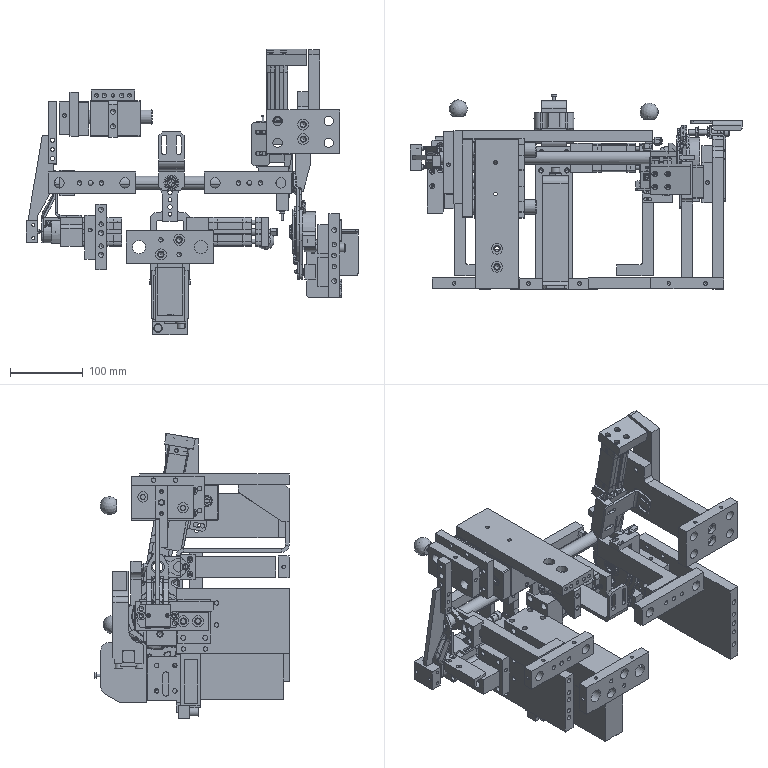Part | NX | features BREP 91 | 136 solids | 8416 faces | volume 4111245 mm3 | plane 3246 | cylinder 3075 | spline 872 | cone 698 | torus 451 | sphere 74 | commonest cylinder face diameters 0.3 x338 0.6 x288 6 x156 1 x140 0.8 x108 2 x92